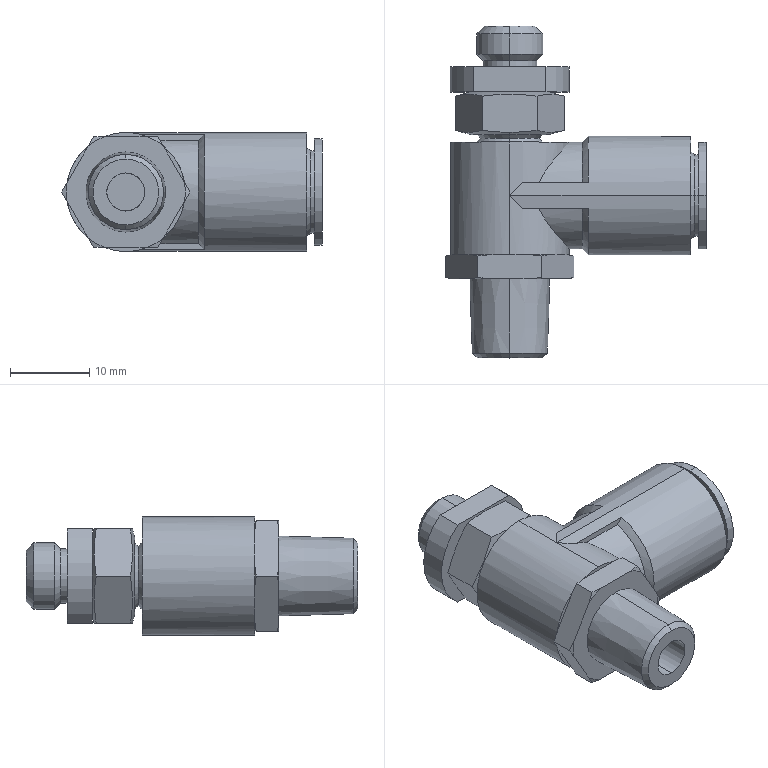Part | STEP file | SPCNL8_1_B_SPCNL8-1-B | 1 solid | 93 faces | box 32.883 x 41.9 x 15 mm | volume 6567 mm3 | plane 36 | cone 32 | cylinder 25 | commonest cylinder face diameters 15 x8 4.8 x5 13.5 x4 6.82 x2 8 x2 8.4 x2